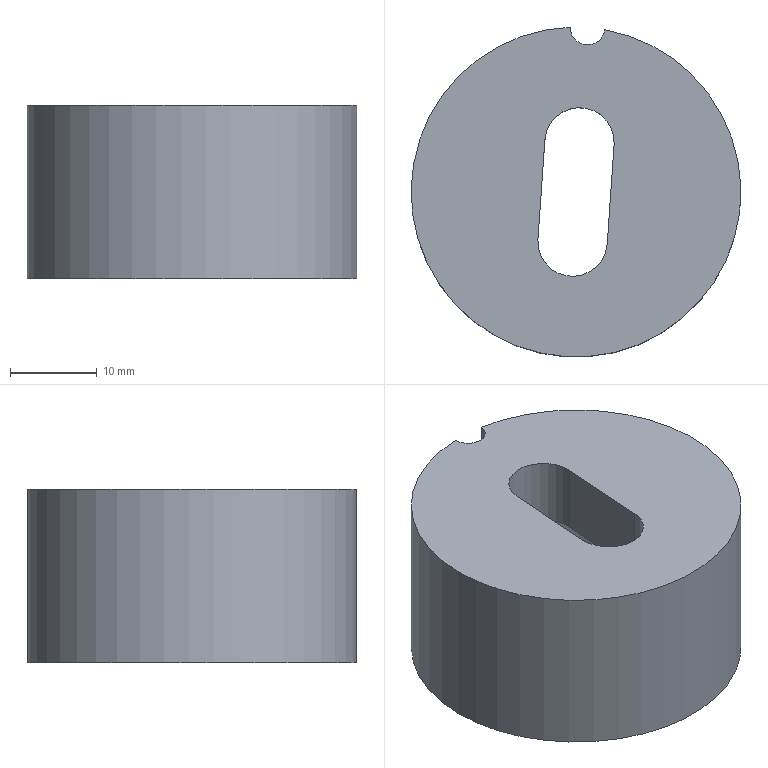Part | NX | features solid 2 | 1 solid | 10 faces | box 38 x 37.988 x 20 mm | volume 14755 mm3 | cylinder 5 | plane 5 | commonest cylinder face diameters 8 x2 4 x1 26.6 x1 38 x1
STEP:
#1=CARTESIAN_POINT('',(626.887,374.134,23.6));
#2=VERTEX_POINT('',#1);
#3=CARTESIAN_POINT('',(625.959,360.867,23.6));
#4=DIRECTION('',(0.,0.,-1.));
#5=DIRECTION('',(0.06976,0.9976,0.));
#6=AXIS2_PLACEMENT_3D('',#3,#4,#5);
#7=CIRCLE('',#6,13.3);
#8=EDGE_CURVE('',#2,#2,#7,.T.);
#9=ORIENTED_EDGE('',*,*,#8,.T.);
#10=EDGE_LOOP('',(#9));
#11=FACE_BOUND('',#10,.T.);
#12=CARTESIAN_POINT('',(612.659,360.867,35.6));
#13=VERTEX_POINT('',#12);
#14=CARTESIAN_POINT('',(625.959,360.867,35.6));
#15=DIRECTION('',(0.,0.,-1.));
#16=DIRECTION('',(-1.,0.,0.));
#17=AXIS2_PLACEMENT_3D('',#14,#15,#16);
#18=CIRCLE('',#17,13.3);
#19=EDGE_CURVE('',#13,#13,#18,.F.);
#20=ORIENTED_EDGE('',*,*,#19,.T.);
#21=EDGE_LOOP('',(#20));
#22=FACE_BOUND('',#21,.T.);
#23=CARTESIAN_POINT('',(625.959,360.867,23.6));
#24=DIRECTION('',(0.,0.,1.));
#25=DIRECTION('',(0.06976,0.9976,0.));
#26=AXIS2_PLACEMENT_3D('',#23,#24,#25);
#27=CYLINDRICAL_SURFACE('',#26,13.3);
#28=ADVANCED_FACE('',(#11,#22),#27,.F.);
#29=CARTESIAN_POINT('',(629.27,379.576,23.6));
#30=VERTEX_POINT('',#29);
#31=CARTESIAN_POINT('',(629.27,379.576,43.6));
#32=VERTEX_POINT('',#31);
#33=CARTESIAN_POINT('',(629.27,379.576,33.6));
#34=DIRECTION('',(0.,0.,1.));
#35=VECTOR('',#34,1000.);
#36=LINE('',#33,#35);
#37=EDGE_CURVE('',#30,#32,#36,.T.);
#38=ORIENTED_EDGE('',*,*,#37,.T.);
#39=CARTESIAN_POINT('',(625.285,379.855,43.6));
#40=VERTEX_POINT('',#39);
#41=CARTESIAN_POINT('',(625.959,360.867,43.6));
#42=DIRECTION('',(0.,0.,-1.));
#43=DIRECTION('',(0.06976,0.9976,0.));
#44=AXIS2_PLACEMENT_3D('',#41,#42,#43);
#45=CIRCLE('',#44,19.);
#46=EDGE_CURVE('',#32,#40,#45,.T.);
#47=ORIENTED_EDGE('',*,*,#46,.T.);
#48=CARTESIAN_POINT('',(625.285,379.855,23.6));
#49=VERTEX_POINT('',#48);
#50=CARTESIAN_POINT('',(625.285,379.855,33.6));
#51=DIRECTION('',(0.,0.,1.));
#52=VECTOR('',#51,1000.);
#53=LINE('',#50,#52);
#54=EDGE_CURVE('',#40,#49,#53,.F.);
#55=ORIENTED_EDGE('',*,*,#54,.T.);
#56=CARTESIAN_POINT('',(625.959,360.867,23.6));
#57=DIRECTION('',(0.,0.,-1.));
#58=DIRECTION('',(0.06976,0.9976,0.));
#59=AXIS2_PLACEMENT_3D('',#56,#57,#58);
#60=CIRCLE('',#59,19.);
#61=EDGE_CURVE('',#30,#49,#60,.T.);
#62=ORIENTED_EDGE('',*,*,#61,.F.);
#63=EDGE_LOOP('',(#38,#47,#55,#62));
#64=FACE_BOUND('',#63,.T.);
#65=CARTESIAN_POINT('',(625.959,360.867,23.6));
#66=DIRECTION('',(0.,0.,1.));
#67=DIRECTION('',(0.06976,0.9976,0.));
#68=AXIS2_PLACEMENT_3D('',#65,#66,#67);
#69=CYLINDRICAL_SURFACE('',#68,19.);
#70=ADVANCED_FACE('',(#64),#69,.T.);
#71=ORIENTED_EDGE('',*,*,#8,.F.);
#72=EDGE_LOOP('',(#71));
#73=FACE_BOUND('',#72,.T.);
#74=ORIENTED_EDGE('',*,*,#61,.T.);
#75=CARTESIAN_POINT('',(627.285,379.82,23.6));
#76=DIRECTION('',(0.,0.,-1.));
#77=DIRECTION('',(0.06976,0.9976,0.));
#78=AXIS2_PLACEMENT_3D('',#75,#76,#77);
#79=CIRCLE('',#78,2.);
#80=EDGE_CURVE('',#30,#49,#79,.T.);
#81=ORIENTED_EDGE('',*,*,#80,.F.);
#82=EDGE_LOOP('',(#74,#81));
#83=FACE_BOUND('',#82,.T.);
#84=CARTESIAN_POINT('',(625.959,360.867,23.6));
#85=DIRECTION('',(0.,0.,1.));
#86=DIRECTION('',(0.06976,0.9976,0.));
#87=AXIS2_PLACEMENT_3D('',#84,#85,#86);
#88=PLANE('',#87);
#89=ADVANCED_FACE('',(#73,#83),#88,.F.);
#90=CARTESIAN_POINT('',(627.285,379.82,43.6));
#91=DIRECTION('',(0.,0.,-1.));
#92=DIRECTION('',(0.06976,0.9976,0.));
#93=AXIS2_PLACEMENT_3D('',#90,#91,#92);
#94=CIRCLE('',#93,2.);
#95=EDGE_CURVE('',#32,#40,#94,.T.);
#96=ORIENTED_EDGE('',*,*,#95,.T.);
#97=ORIENTED_EDGE('',*,*,#46,.F.);
#98=EDGE_LOOP('',(#96,#97));
#99=FACE_BOUND('',#98,.T.);
#100=CARTESIAN_POINT('',(621.569,355.425,43.6));
#101=VERTEX_POINT('',#100);
#102=CARTESIAN_POINT('',(622.369,366.867,43.6));
#103=VERTEX_POINT('',#102);
#104=CARTESIAN_POINT('',(621.569,355.425,43.6));
#105=DIRECTION('',(0.06976,0.9976,0.));
#106=VECTOR('',#105,1000.);
#107=LINE('',#104,#106);
#108=EDGE_CURVE('',#101,#103,#107,.T.);
#109=ORIENTED_EDGE('',*,*,#108,.T.);
#110=CARTESIAN_POINT('',(630.35,366.309,43.6));
#111=VERTEX_POINT('',#110);
#112=CARTESIAN_POINT('',(626.359,366.588,43.6));
#113=DIRECTION('',(0.,0.,-1.));
#114=DIRECTION('',(0.9976,-0.06976,0.));
#115=AXIS2_PLACEMENT_3D('',#112,#113,#114);
#116=CIRCLE('',#115,4.);
#117=EDGE_CURVE('',#103,#111,#116,.T.);
#118=ORIENTED_EDGE('',*,*,#117,.T.);
#119=CARTESIAN_POINT('',(629.55,354.866,43.6));
#120=VERTEX_POINT('',#119);
#121=CARTESIAN_POINT('',(629.55,354.866,43.6));
#122=DIRECTION('',(0.06976,0.9976,0.));
#123=VECTOR('',#122,1000.);
#124=LINE('',#121,#123);
#125=EDGE_CURVE('',#120,#111,#124,.T.);
#126=ORIENTED_EDGE('',*,*,#125,.F.);
#127=CARTESIAN_POINT('',(625.559,355.146,43.6));
#128=DIRECTION('',(0.,0.,-1.));
#129=DIRECTION('',(0.9976,-0.06976,0.));
#130=AXIS2_PLACEMENT_3D('',#127,#128,#129);
#131=CIRCLE('',#130,4.);
#132=EDGE_CURVE('',#120,#101,#131,.T.);
#133=ORIENTED_EDGE('',*,*,#132,.T.);
#134=EDGE_LOOP('',(#109,#118,#126,#133));
#135=FACE_BOUND('',#134,.T.);
#136=CARTESIAN_POINT('',(625.959,360.867,43.6));
#137=DIRECTION('',(0.,0.,1.));
#138=DIRECTION('',(0.06976,0.9976,0.));
#139=AXIS2_PLACEMENT_3D('',#136,#137,#138);
#140=PLANE('',#139);
#141=ADVANCED_FACE('',(#99,#135),#140,.T.);
#142=ORIENTED_EDGE('',*,*,#37,.F.);
#143=ORIENTED_EDGE('',*,*,#80,.T.);
#144=ORIENTED_EDGE('',*,*,#54,.F.);
#145=ORIENTED_EDGE('',*,*,#95,.F.);
#146=EDGE_LOOP('',(#142,#143,#144,#145));
#147=FACE_BOUND('',#146,.T.);
#148=CARTESIAN_POINT('',(627.285,379.82,23.6));
#149=DIRECTION('',(0.,0.,1.));
#150=DIRECTION('',(0.06976,0.9976,0.));
#151=AXIS2_PLACEMENT_3D('',#148,#149,#150);
#152=CYLINDRICAL_SURFACE('',#151,2.);
#153=ADVANCED_FACE('',(#147),#152,.F.);
#154=CARTESIAN_POINT('',(629.55,354.866,35.6));
#155=VERTEX_POINT('',#154);
#156=CARTESIAN_POINT('',(630.35,366.309,35.6));
#157=VERTEX_POINT('',#156);
#158=CARTESIAN_POINT('',(629.95,360.588,35.6));
#159=DIRECTION('',(0.06976,0.9976,0.));
#160=VECTOR('',#159,1000.);
#161=LINE('',#158,#160);
#162=EDGE_CURVE('',#155,#157,#161,.T.);
#163=ORIENTED_EDGE('',*,*,#162,.F.);
#164=CARTESIAN_POINT('',(629.55,354.866,23.6));
#165=DIRECTION('',(0.,0.,1.));
#166=VECTOR('',#165,1000.);
#167=LINE('',#164,#166);
#168=EDGE_CURVE('',#155,#120,#167,.T.);
#169=ORIENTED_EDGE('',*,*,#168,.T.);
#170=ORIENTED_EDGE('',*,*,#125,.T.);
#171=CARTESIAN_POINT('',(630.35,366.309,23.6));
#172=DIRECTION('',(0.,0.,1.));
#173=VECTOR('',#172,1000.);
#174=LINE('',#171,#173);
#175=EDGE_CURVE('',#157,#111,#174,.T.);
#176=ORIENTED_EDGE('',*,*,#175,.F.);
#177=EDGE_LOOP('',(#163,#169,#170,#176));
#178=FACE_BOUND('',#177,.T.);
#179=CARTESIAN_POINT('',(629.55,354.866,23.6));
#180=DIRECTION('',(-0.9976,0.06976,0.));
#181=DIRECTION('',(0.,0.,1.));
#182=AXIS2_PLACEMENT_3D('',#179,#180,#181);
#183=PLANE('',#182);
#184=ADVANCED_FACE('',(#178),#183,.T.);
#185=CARTESIAN_POINT('',(622.369,366.867,35.6));
#186=VERTEX_POINT('',#185);
#187=CARTESIAN_POINT('',(622.369,366.867,23.6));
#188=DIRECTION('',(0.,0.,1.));
#189=VECTOR('',#188,1000.);
#190=LINE('',#187,#189);
#191=EDGE_CURVE('',#186,#103,#190,.T.);
#192=ORIENTED_EDGE('',*,*,#191,.F.);
#193=CARTESIAN_POINT('',(626.359,366.588,35.6));
#194=DIRECTION('',(0.,0.,-1.));
#195=DIRECTION('',(0.9976,-0.06976,0.));
#196=AXIS2_PLACEMENT_3D('',#193,#194,#195);
#197=CIRCLE('',#196,4.);
#198=EDGE_CURVE('',#186,#157,#197,.T.);
#199=ORIENTED_EDGE('',*,*,#198,.T.);
#200=ORIENTED_EDGE('',*,*,#175,.T.);
#201=ORIENTED_EDGE('',*,*,#117,.F.);
#202=EDGE_LOOP('',(#192,#199,#200,#201));
#203=FACE_BOUND('',#202,.T.);
#204=CARTESIAN_POINT('',(626.359,366.588,23.6));
#205=DIRECTION('',(0.,0.,1.));
#206=DIRECTION('',(0.9976,-0.06976,0.));
#207=AXIS2_PLACEMENT_3D('',#204,#205,#206);
#208=CYLINDRICAL_SURFACE('',#207,4.);
#209=ADVANCED_FACE('',(#203),#208,.F.);
#210=CARTESIAN_POINT('',(621.569,355.425,35.6));
#211=VERTEX_POINT('',#210);
#212=CARTESIAN_POINT('',(621.569,355.425,23.6));
#213=DIRECTION('',(0.,0.,1.));
#214=VECTOR('',#213,1000.);
#215=LINE('',#212,#214);
#216=EDGE_CURVE('',#211,#101,#215,.T.);
#217=ORIENTED_EDGE('',*,*,#216,.F.);
#218=CARTESIAN_POINT('',(621.969,361.146,35.6));
#219=DIRECTION('',(0.06976,0.9976,0.));
#220=VECTOR('',#219,1000.);
#221=LINE('',#218,#220);
#222=EDGE_CURVE('',#211,#186,#221,.T.);
#223=ORIENTED_EDGE('',*,*,#222,.T.);
#224=ORIENTED_EDGE('',*,*,#191,.T.);
#225=ORIENTED_EDGE('',*,*,#108,.F.);
#226=EDGE_LOOP('',(#217,#223,#224,#225));
#227=FACE_BOUND('',#226,.T.);
#228=CARTESIAN_POINT('',(621.569,355.425,23.6));
#229=DIRECTION('',(-0.9976,0.06976,0.));
#230=DIRECTION('',(0.,0.,1.));
#231=AXIS2_PLACEMENT_3D('',#228,#229,#230);
#232=PLANE('',#231);
#233=ADVANCED_FACE('',(#227),#232,.F.);
#234=ORIENTED_EDGE('',*,*,#168,.F.);
#235=CARTESIAN_POINT('',(625.559,355.146,35.6));
#236=DIRECTION('',(0.,0.,-1.));
#237=DIRECTION('',(0.9976,-0.06976,0.));
#238=AXIS2_PLACEMENT_3D('',#235,#236,#237);
#239=CIRCLE('',#238,4.);
#240=EDGE_CURVE('',#155,#211,#239,.T.);
#241=ORIENTED_EDGE('',*,*,#240,.T.);
#242=ORIENTED_EDGE('',*,*,#216,.T.);
#243=ORIENTED_EDGE('',*,*,#132,.F.);
#244=EDGE_LOOP('',(#234,#241,#242,#243));
#245=FACE_BOUND('',#244,.T.);
#246=CARTESIAN_POINT('',(625.559,355.146,23.6));
#247=DIRECTION('',(0.,0.,1.));
#248=DIRECTION('',(0.9976,-0.06976,0.));
#249=AXIS2_PLACEMENT_3D('',#246,#247,#248);
#250=CYLINDRICAL_SURFACE('',#249,4.);
#251=ADVANCED_FACE('',(#245),#250,.F.);
#252=ORIENTED_EDGE('',*,*,#240,.F.);
#253=ORIENTED_EDGE('',*,*,#162,.T.);
#254=ORIENTED_EDGE('',*,*,#198,.F.);
#255=ORIENTED_EDGE('',*,*,#222,.F.);
#256=EDGE_LOOP('',(#252,#253,#254,#255));
#257=FACE_BOUND('',#256,.T.);
#258=ORIENTED_EDGE('',*,*,#19,.F.);
#259=EDGE_LOOP('',(#258));
#260=FACE_BOUND('',#259,.T.);
#261=CARTESIAN_POINT('',(625.959,360.867,35.6));
#262=DIRECTION('',(0.,0.,1.));
#263=DIRECTION('',(0.9976,-0.06976,0.));
#264=AXIS2_PLACEMENT_3D('',#261,#262,#263);
#265=PLANE('',#264);
#266=ADVANCED_FACE('',(#257,#260),#265,.F.);
#267=CLOSED_SHELL('',(#28,#70,#89,#141,#153,#184,#209,#233,#251,#266));
#268=MANIFOLD_SOLID_BREP('',#267);
#269=(LENGTH_UNIT()NAMED_UNIT(*)SI_UNIT(.MILLI.,.METRE.));
#270=UNCERTAINTY_MEASURE_WITH_UNIT(LENGTH_MEASURE(0.00001),#269,'','');
#271=(NAMED_UNIT(*)PLANE_ANGLE_UNIT()SI_UNIT($,.RADIAN.));
#272=(NAMED_UNIT(*)SI_UNIT($,.STERADIAN.)SOLID_ANGLE_UNIT());
#273=(GEOMETRIC_REPRESENTATION_CONTEXT(3)GLOBAL_UNCERTAINTY_ASSIGNED_CONTEXT((#270))GLOBAL_UNIT_ASSIGNED_CONTEXT((#269,#271,#272))REPRESENTATION_CONTEXT('',''));
#274=ADVANCED_BREP_SHAPE_REPRESENTATION('',(#268),#273);